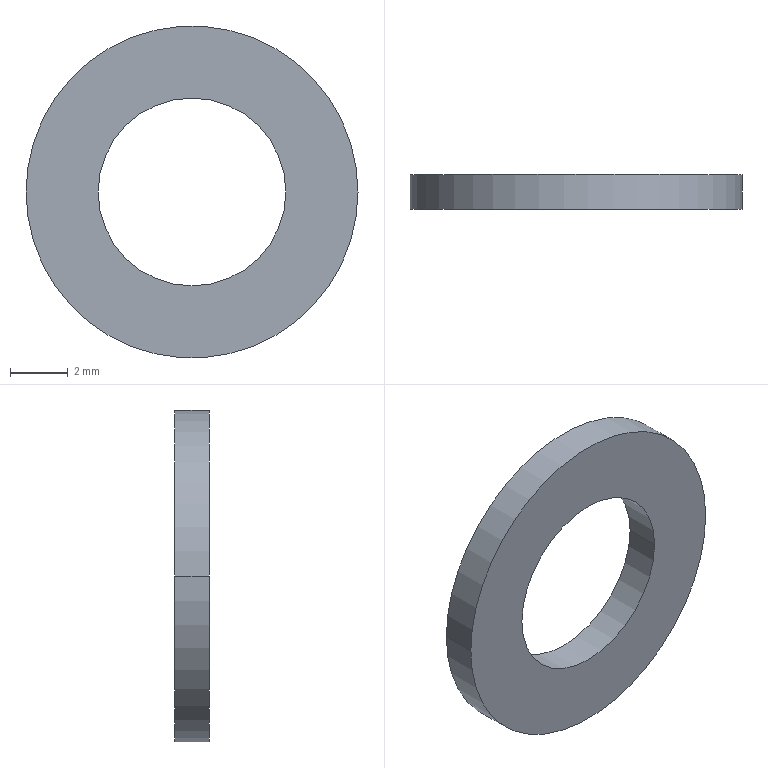Part | STEP file | WSX-SUS-M6X11.5-1.2-5 | 1 solid | 6 faces | box 11.5 x 1.2 x 11.5 mm | volume 84.823 mm3 | cylinder 4 | plane 2 | commonest cylinder face diameters 6.5 x2 11.5 x2
STEP:
#1=CARTESIAN_POINT('',(3.25,1.2,0.));
#2=VERTEX_POINT('',#1);
#3=CARTESIAN_POINT('',(-3.25,1.2,0.));
#4=VERTEX_POINT('',#3);
#5=CARTESIAN_POINT('',(0.,1.2,0.));
#6=DIRECTION('',(0.,-1.,0.));
#7=DIRECTION('',(-1.,0.,0.));
#8=AXIS2_PLACEMENT_3D('',#5,#6,#7);
#9=CIRCLE('',#8,3.25);
#10=EDGE_CURVE('',#2,#4,#9,.T.);
#11=ORIENTED_EDGE('',*,*,#10,.F.);
#12=CARTESIAN_POINT('',(3.25,0.,0.));
#13=VERTEX_POINT('',#12);
#14=CARTESIAN_POINT('',(3.25,1.2,0.));
#15=DIRECTION('',(0.,-1.,0.));
#16=VECTOR('',#15,1000.);
#17=LINE('',#14,#16);
#18=EDGE_CURVE('',#2,#13,#17,.T.);
#19=ORIENTED_EDGE('',*,*,#18,.T.);
#20=CARTESIAN_POINT('',(-3.25,0.,0.));
#21=VERTEX_POINT('',#20);
#22=CARTESIAN_POINT('',(0.,0.,0.));
#23=DIRECTION('',(0.,1.,0.));
#24=DIRECTION('',(1.,0.,0.));
#25=AXIS2_PLACEMENT_3D('',#22,#23,#24);
#26=CIRCLE('',#25,3.25);
#27=EDGE_CURVE('',#21,#13,#26,.T.);
#28=ORIENTED_EDGE('',*,*,#27,.F.);
#29=CARTESIAN_POINT('',(-3.25,1.2,0.));
#30=DIRECTION('',(0.,-1.,0.));
#31=VECTOR('',#30,1000.);
#32=LINE('',#29,#31);
#33=EDGE_CURVE('',#4,#21,#32,.T.);
#34=ORIENTED_EDGE('',*,*,#33,.F.);
#35=EDGE_LOOP('',(#11,#19,#28,#34));
#36=FACE_OUTER_BOUND('',#35,.T.);
#37=CARTESIAN_POINT('',(0.,1.2,0.));
#38=DIRECTION('',(0.,-1.,0.));
#39=DIRECTION('',(-1.,0.,0.));
#40=AXIS2_PLACEMENT_3D('',#37,#38,#39);
#41=CYLINDRICAL_SURFACE('',#40,3.25);
#42=ADVANCED_FACE('',(#36),#41,.F.);
#43=CARTESIAN_POINT('',(-5.75,1.2,0.));
#44=VERTEX_POINT('',#43);
#45=CARTESIAN_POINT('',(5.75,1.2,0.));
#46=VERTEX_POINT('',#45);
#47=CARTESIAN_POINT('',(0.,1.2,0.));
#48=DIRECTION('',(0.,-1.,0.));
#49=DIRECTION('',(-1.,0.,0.));
#50=AXIS2_PLACEMENT_3D('',#47,#48,#49);
#51=CIRCLE('',#50,5.75);
#52=EDGE_CURVE('',#44,#46,#51,.T.);
#53=ORIENTED_EDGE('',*,*,#52,.T.);
#54=CARTESIAN_POINT('',(5.75,0.,0.));
#55=VERTEX_POINT('',#54);
#56=CARTESIAN_POINT('',(5.75,1.2,0.));
#57=DIRECTION('',(0.,-1.,0.));
#58=VECTOR('',#57,1000.);
#59=LINE('',#56,#58);
#60=EDGE_CURVE('',#46,#55,#59,.T.);
#61=ORIENTED_EDGE('',*,*,#60,.T.);
#62=CARTESIAN_POINT('',(-5.75,0.,0.));
#63=VERTEX_POINT('',#62);
#64=CARTESIAN_POINT('',(0.,0.,0.));
#65=DIRECTION('',(0.,1.,0.));
#66=DIRECTION('',(1.,0.,0.));
#67=AXIS2_PLACEMENT_3D('',#64,#65,#66);
#68=CIRCLE('',#67,5.75);
#69=EDGE_CURVE('',#55,#63,#68,.T.);
#70=ORIENTED_EDGE('',*,*,#69,.T.);
#71=CARTESIAN_POINT('',(-5.75,1.2,0.));
#72=DIRECTION('',(0.,-1.,0.));
#73=VECTOR('',#72,1000.);
#74=LINE('',#71,#73);
#75=EDGE_CURVE('',#44,#63,#74,.T.);
#76=ORIENTED_EDGE('',*,*,#75,.F.);
#77=EDGE_LOOP('',(#53,#61,#70,#76));
#78=FACE_OUTER_BOUND('',#77,.T.);
#79=CARTESIAN_POINT('',(0.,1.2,0.));
#80=DIRECTION('',(0.,-1.,0.));
#81=DIRECTION('',(-1.,0.,0.));
#82=AXIS2_PLACEMENT_3D('',#79,#80,#81);
#83=CYLINDRICAL_SURFACE('',#82,5.75);
#84=ADVANCED_FACE('',(#78),#83,.T.);
#85=ORIENTED_EDGE('',*,*,#27,.T.);
#86=CARTESIAN_POINT('',(0.,0.,0.));
#87=DIRECTION('',(0.,1.,0.));
#88=DIRECTION('',(1.,0.,0.));
#89=AXIS2_PLACEMENT_3D('',#86,#87,#88);
#90=CIRCLE('',#89,3.25);
#91=EDGE_CURVE('',#13,#21,#90,.T.);
#92=ORIENTED_EDGE('',*,*,#91,.T.);
#93=EDGE_LOOP('',(#85,#92));
#94=FACE_BOUND('',#93,.T.);
#95=CARTESIAN_POINT('',(0.,0.,0.));
#96=DIRECTION('',(0.,1.,0.));
#97=DIRECTION('',(1.,0.,0.));
#98=AXIS2_PLACEMENT_3D('',#95,#96,#97);
#99=CIRCLE('',#98,5.75);
#100=EDGE_CURVE('',#63,#55,#99,.T.);
#101=ORIENTED_EDGE('',*,*,#100,.F.);
#102=ORIENTED_EDGE('',*,*,#69,.F.);
#103=EDGE_LOOP('',(#101,#102));
#104=FACE_OUTER_BOUND('',#103,.T.);
#105=CARTESIAN_POINT('',(0.,0.,0.));
#106=DIRECTION('',(0.,-1.,0.));
#107=DIRECTION('',(-1.,0.,0.));
#108=AXIS2_PLACEMENT_3D('',#105,#106,#107);
#109=PLANE('',#108);
#110=ADVANCED_FACE('',(#94,#104),#109,.T.);
#111=CARTESIAN_POINT('',(0.,1.2,0.));
#112=DIRECTION('',(0.,-1.,0.));
#113=DIRECTION('',(-1.,0.,0.));
#114=AXIS2_PLACEMENT_3D('',#111,#112,#113);
#115=CIRCLE('',#114,3.25);
#116=EDGE_CURVE('',#4,#2,#115,.T.);
#117=ORIENTED_EDGE('',*,*,#116,.T.);
#118=ORIENTED_EDGE('',*,*,#10,.T.);
#119=EDGE_LOOP('',(#117,#118));
#120=FACE_BOUND('',#119,.T.);
#121=ORIENTED_EDGE('',*,*,#52,.F.);
#122=CARTESIAN_POINT('',(0.,1.2,0.));
#123=DIRECTION('',(0.,-1.,0.));
#124=DIRECTION('',(-1.,0.,0.));
#125=AXIS2_PLACEMENT_3D('',#122,#123,#124);
#126=CIRCLE('',#125,5.75);
#127=EDGE_CURVE('',#46,#44,#126,.T.);
#128=ORIENTED_EDGE('',*,*,#127,.F.);
#129=EDGE_LOOP('',(#121,#128));
#130=FACE_OUTER_BOUND('',#129,.T.);
#131=CARTESIAN_POINT('',(0.,1.2,0.));
#132=DIRECTION('',(0.,1.,0.));
#133=DIRECTION('',(1.,0.,0.));
#134=AXIS2_PLACEMENT_3D('',#131,#132,#133);
#135=PLANE('',#134);
#136=ADVANCED_FACE('',(#120,#130),#135,.T.);
#137=ORIENTED_EDGE('',*,*,#60,.F.);
#138=ORIENTED_EDGE('',*,*,#127,.T.);
#139=ORIENTED_EDGE('',*,*,#75,.T.);
#140=ORIENTED_EDGE('',*,*,#100,.T.);
#141=EDGE_LOOP('',(#137,#138,#139,#140));
#142=FACE_OUTER_BOUND('',#141,.T.);
#143=CARTESIAN_POINT('',(0.,1.2,0.));
#144=DIRECTION('',(0.,-1.,0.));
#145=DIRECTION('',(-1.,0.,0.));
#146=AXIS2_PLACEMENT_3D('',#143,#144,#145);
#147=CYLINDRICAL_SURFACE('',#146,5.75);
#148=ADVANCED_FACE('',(#142),#147,.T.);
#149=ORIENTED_EDGE('',*,*,#18,.F.);
#150=ORIENTED_EDGE('',*,*,#116,.F.);
#151=ORIENTED_EDGE('',*,*,#33,.T.);
#152=ORIENTED_EDGE('',*,*,#91,.F.);
#153=EDGE_LOOP('',(#149,#150,#151,#152));
#154=FACE_OUTER_BOUND('',#153,.T.);
#155=CARTESIAN_POINT('',(0.,1.2,0.));
#156=DIRECTION('',(0.,-1.,0.));
#157=DIRECTION('',(-1.,0.,0.));
#158=AXIS2_PLACEMENT_3D('',#155,#156,#157);
#159=CYLINDRICAL_SURFACE('',#158,3.25);
#160=ADVANCED_FACE('',(#154),#159,.F.);
#161=CLOSED_SHELL('',(#42,#84,#110,#136,#148,#160));
#162=MANIFOLD_SOLID_BREP('',#161);
#163=CARTESIAN_POINT('',(0.,0.,0.));
#164=DIRECTION('',(0.,0.,1.));
#165=DIRECTION('',(1.,0.,0.));
#166=AXIS2_PLACEMENT_3D('',#163,#164,#165);
#167=(LENGTH_UNIT()NAMED_UNIT(*)SI_UNIT(.MILLI.,.METRE.));
#168=UNCERTAINTY_MEASURE_WITH_UNIT(LENGTH_MEASURE(0.00001),#167,'','');
#169=(NAMED_UNIT(*)PLANE_ANGLE_UNIT()SI_UNIT($,.RADIAN.));
#170=(NAMED_UNIT(*)SI_UNIT($,.STERADIAN.)SOLID_ANGLE_UNIT());
#171=(GEOMETRIC_REPRESENTATION_CONTEXT(3)GLOBAL_UNCERTAINTY_ASSIGNED_CONTEXT((#168))GLOBAL_UNIT_ASSIGNED_CONTEXT((#167,#169,#170))REPRESENTATION_CONTEXT('',''));
#172=ADVANCED_BREP_SHAPE_REPRESENTATION('',(#162,#166),#171);